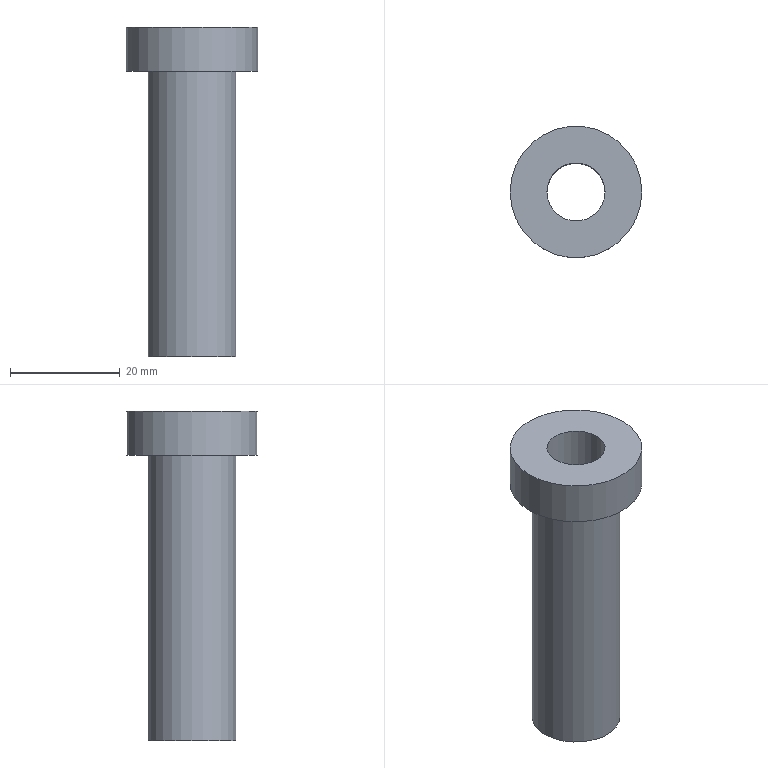Part | NX | features solid 2 | 1 solid | 6 faces | box 24 x 24 x 60 mm | volume 8779 mm3 | plane 3 | cylinder 3 | commonest cylinder face diameters 10.6 x1 16 x1 24 x1
STEP:
#1=CARTESIAN_POINT('',(-1461.255,409.161,32.));
#2=VERTEX_POINT('',#1);
#3=CARTESIAN_POINT('',(-1473.255,409.161,32.));
#4=DIRECTION('',(0.,0.,-1.));
#5=DIRECTION('',(1.,0.,0.));
#6=AXIS2_PLACEMENT_3D('',#3,#4,#5);
#7=CIRCLE('',#6,12.);
#8=EDGE_CURVE('',#2,#2,#7,.F.);
#9=ORIENTED_EDGE('',*,*,#8,.F.);
#10=EDGE_LOOP('',(#9));
#11=FACE_BOUND('',#10,.T.);
#12=CARTESIAN_POINT('',(-1481.255,409.161,32.));
#13=VERTEX_POINT('',#12);
#14=CARTESIAN_POINT('',(-1473.255,409.161,32.));
#15=DIRECTION('',(0.,0.,1.));
#16=DIRECTION('',(-1.,0.,0.));
#17=AXIS2_PLACEMENT_3D('',#14,#15,#16);
#18=CIRCLE('',#17,8.);
#19=EDGE_CURVE('',#13,#13,#18,.T.);
#20=ORIENTED_EDGE('',*,*,#19,.T.);
#21=EDGE_LOOP('',(#20));
#22=FACE_BOUND('',#21,.T.);
#23=CARTESIAN_POINT('',(-1473.255,409.161,32.));
#24=DIRECTION('',(0.,0.,-1.));
#25=DIRECTION('',(-1.,0.,0.));
#26=AXIS2_PLACEMENT_3D('',#23,#24,#25);
#27=PLANE('',#26);
#28=ADVANCED_FACE('',(#11,#22),#27,.T.);
#29=CARTESIAN_POINT('',(-1467.955,409.161,40.));
#30=VERTEX_POINT('',#29);
#31=CARTESIAN_POINT('',(-1473.255,409.161,40.));
#32=DIRECTION('',(0.,0.,-1.));
#33=DIRECTION('',(1.,0.,0.));
#34=AXIS2_PLACEMENT_3D('',#31,#32,#33);
#35=CIRCLE('',#34,5.3);
#36=EDGE_CURVE('',#30,#30,#35,.T.);
#37=ORIENTED_EDGE('',*,*,#36,.T.);
#38=EDGE_LOOP('',(#37));
#39=FACE_BOUND('',#38,.T.);
#40=CARTESIAN_POINT('',(-1461.255,409.161,40.));
#41=VERTEX_POINT('',#40);
#42=CARTESIAN_POINT('',(-1473.255,409.161,40.));
#43=DIRECTION('',(0.,0.,-1.));
#44=DIRECTION('',(1.,0.,0.));
#45=AXIS2_PLACEMENT_3D('',#42,#43,#44);
#46=CIRCLE('',#45,12.);
#47=EDGE_CURVE('',#41,#41,#46,.F.);
#48=ORIENTED_EDGE('',*,*,#47,.T.);
#49=EDGE_LOOP('',(#48));
#50=FACE_BOUND('',#49,.T.);
#51=CARTESIAN_POINT('',(-1473.255,409.161,40.));
#52=DIRECTION('',(0.,0.,-1.));
#53=DIRECTION('',(-1.,0.,0.));
#54=AXIS2_PLACEMENT_3D('',#51,#52,#53);
#55=PLANE('',#54);
#56=ADVANCED_FACE('',(#39,#50),#55,.F.);
#57=ORIENTED_EDGE('',*,*,#47,.F.);
#58=EDGE_LOOP('',(#57));
#59=FACE_BOUND('',#58,.T.);
#60=ORIENTED_EDGE('',*,*,#8,.T.);
#61=EDGE_LOOP('',(#60));
#62=FACE_BOUND('',#61,.T.);
#63=CARTESIAN_POINT('',(-1473.255,409.161,32.));
#64=DIRECTION('',(0.,0.,1.));
#65=DIRECTION('',(1.,0.,0.));
#66=AXIS2_PLACEMENT_3D('',#63,#64,#65);
#67=CYLINDRICAL_SURFACE('',#66,12.);
#68=ADVANCED_FACE('',(#59,#62),#67,.T.);
#69=CARTESIAN_POINT('',(-1467.955,409.161,-20.));
#70=VERTEX_POINT('',#69);
#71=CARTESIAN_POINT('',(-1473.255,409.161,-20.));
#72=DIRECTION('',(0.,0.,-1.));
#73=DIRECTION('',(1.,0.,0.));
#74=AXIS2_PLACEMENT_3D('',#71,#72,#73);
#75=CIRCLE('',#74,5.3);
#76=EDGE_CURVE('',#70,#70,#75,.F.);
#77=ORIENTED_EDGE('',*,*,#76,.T.);
#78=EDGE_LOOP('',(#77));
#79=FACE_BOUND('',#78,.T.);
#80=CARTESIAN_POINT('',(-1465.255,409.161,-20.));
#81=VERTEX_POINT('',#80);
#82=CARTESIAN_POINT('',(-1473.255,409.161,-20.));
#83=DIRECTION('',(0.,0.,-1.));
#84=DIRECTION('',(1.,0.,0.));
#85=AXIS2_PLACEMENT_3D('',#82,#83,#84);
#86=CIRCLE('',#85,8.);
#87=EDGE_CURVE('',#81,#81,#86,.F.);
#88=ORIENTED_EDGE('',*,*,#87,.F.);
#89=EDGE_LOOP('',(#88));
#90=FACE_BOUND('',#89,.T.);
#91=CARTESIAN_POINT('',(-1473.255,409.161,-20.));
#92=DIRECTION('',(0.,0.,-1.));
#93=DIRECTION('',(-1.,0.,0.));
#94=AXIS2_PLACEMENT_3D('',#91,#92,#93);
#95=PLANE('',#94);
#96=ADVANCED_FACE('',(#79,#90),#95,.T.);
#97=ORIENTED_EDGE('',*,*,#87,.T.);
#98=EDGE_LOOP('',(#97));
#99=FACE_BOUND('',#98,.T.);
#100=ORIENTED_EDGE('',*,*,#19,.F.);
#101=EDGE_LOOP('',(#100));
#102=FACE_BOUND('',#101,.T.);
#103=CARTESIAN_POINT('',(-1473.255,409.161,26.5));
#104=DIRECTION('',(0.,0.,1.));
#105=DIRECTION('',(0.,1.,0.));
#106=AXIS2_PLACEMENT_3D('',#103,#104,#105);
#107=CYLINDRICAL_SURFACE('',#106,8.);
#108=ADVANCED_FACE('',(#99,#102),#107,.T.);
#109=ORIENTED_EDGE('',*,*,#36,.F.);
#110=EDGE_LOOP('',(#109));
#111=FACE_BOUND('',#110,.T.);
#112=ORIENTED_EDGE('',*,*,#76,.F.);
#113=EDGE_LOOP('',(#112));
#114=FACE_BOUND('',#113,.T.);
#115=CARTESIAN_POINT('',(-1473.255,409.161,40.));
#116=DIRECTION('',(0.,0.,-1.));
#117=DIRECTION('',(1.,0.,0.));
#118=AXIS2_PLACEMENT_3D('',#115,#116,#117);
#119=CYLINDRICAL_SURFACE('',#118,5.3);
#120=ADVANCED_FACE('',(#111,#114),#119,.F.);
#121=CLOSED_SHELL('',(#28,#56,#68,#96,#108,#120));
#122=MANIFOLD_SOLID_BREP('',#121);
#123=(LENGTH_UNIT()NAMED_UNIT(*)SI_UNIT(.MILLI.,.METRE.));
#124=UNCERTAINTY_MEASURE_WITH_UNIT(LENGTH_MEASURE(0.00001),#123,'','');
#125=(NAMED_UNIT(*)PLANE_ANGLE_UNIT()SI_UNIT($,.RADIAN.));
#126=(NAMED_UNIT(*)SI_UNIT($,.STERADIAN.)SOLID_ANGLE_UNIT());
#127=(GEOMETRIC_REPRESENTATION_CONTEXT(3)GLOBAL_UNCERTAINTY_ASSIGNED_CONTEXT((#124))GLOBAL_UNIT_ASSIGNED_CONTEXT((#123,#125,#126))REPRESENTATION_CONTEXT('',''));
#128=ADVANCED_BREP_SHAPE_REPRESENTATION('',(#122),#127);